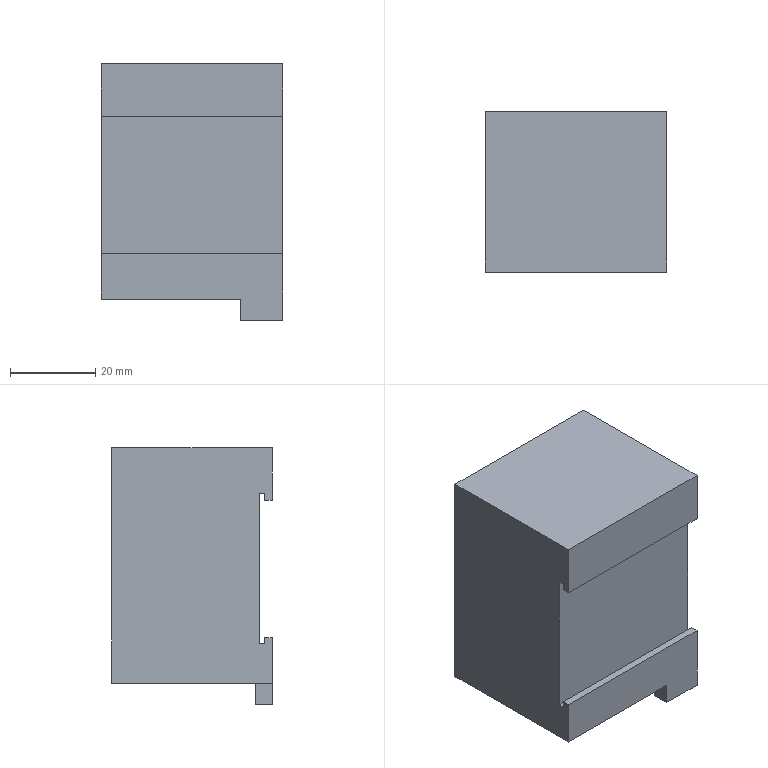Part | SolidWorks | features Cut 1, Extrusion 1, ICE 1 | 1 solid | 17 faces | box 42.7 x 37.7 x 60.3 mm | volume 84935 mm3 | plane 17
STEP:
#1=CARTESIAN_POINT('',(-21.35,0.,15.25));
#2=VERTEX_POINT('',#1);
#3=CARTESIAN_POINT('',(-21.35,0.,27.65));
#4=VERTEX_POINT('',#3);
#5=CARTESIAN_POINT('',(-21.35,0.,27.65));
#6=DIRECTION('',(0.,0.,1.));
#7=VECTOR('',#6,1000.);
#8=LINE('',#5,#7);
#9=EDGE_CURVE('',#2,#4,#8,.T.);
#10=ORIENTED_EDGE('',*,*,#9,.F.);
#11=CARTESIAN_POINT('',(21.35,0.,15.25));
#12=VERTEX_POINT('',#11);
#13=CARTESIAN_POINT('',(-21.351,0.,15.25));
#14=DIRECTION('',(1.,0.,0.));
#15=VECTOR('',#14,1000.);
#16=LINE('',#13,#15);
#17=EDGE_CURVE('',#2,#12,#16,.T.);
#18=ORIENTED_EDGE('',*,*,#17,.T.);
#19=CARTESIAN_POINT('',(21.35,0.,27.65));
#20=VERTEX_POINT('',#19);
#21=CARTESIAN_POINT('',(21.35,0.,27.65));
#22=DIRECTION('',(0.,0.,-1.));
#23=VECTOR('',#22,1000.);
#24=LINE('',#21,#23);
#25=EDGE_CURVE('',#20,#12,#24,.T.);
#26=ORIENTED_EDGE('',*,*,#25,.F.);
#27=CARTESIAN_POINT('',(-21.35,0.,27.65));
#28=DIRECTION('',(1.,0.,0.));
#29=VECTOR('',#28,1000.);
#30=LINE('',#27,#29);
#31=EDGE_CURVE('',#4,#20,#30,.T.);
#32=ORIENTED_EDGE('',*,*,#31,.F.);
#33=EDGE_LOOP('',(#10,#18,#26,#32));
#34=FACE_OUTER_BOUND('',#33,.T.);
#35=CARTESIAN_POINT('',(0.,0.,0.));
#36=DIRECTION('',(0.,-1.,0.));
#37=DIRECTION('',(0.,0.,-1.));
#38=AXIS2_PLACEMENT_3D('',#35,#36,#37);
#39=PLANE('',#38);
#40=ADVANCED_FACE('',(#34),#39,.T.);
#41=CARTESIAN_POINT('',(21.35,0.,-16.95));
#42=VERTEX_POINT('',#41);
#43=CARTESIAN_POINT('',(21.35,1.8,-16.95));
#44=VERTEX_POINT('',#43);
#45=CARTESIAN_POINT('',(21.35,1.8,-16.95));
#46=DIRECTION('',(0.,1.,0.));
#47=VECTOR('',#46,1000.);
#48=LINE('',#45,#47);
#49=EDGE_CURVE('',#42,#44,#48,.T.);
#50=ORIENTED_EDGE('',*,*,#49,.F.);
#51=CARTESIAN_POINT('',(21.35,0.,-32.65));
#52=VERTEX_POINT('',#51);
#53=CARTESIAN_POINT('',(21.35,0.,27.65));
#54=DIRECTION('',(0.,0.,-1.));
#55=VECTOR('',#54,1000.);
#56=LINE('',#53,#55);
#57=EDGE_CURVE('',#42,#52,#56,.T.);
#58=ORIENTED_EDGE('',*,*,#57,.T.);
#59=CARTESIAN_POINT('',(21.35,4.,-32.65));
#60=VERTEX_POINT('',#59);
#61=CARTESIAN_POINT('',(21.35,4.,-32.65));
#62=DIRECTION('',(0.,-1.,0.));
#63=VECTOR('',#62,1000.);
#64=LINE('',#61,#63);
#65=EDGE_CURVE('',#60,#52,#64,.T.);
#66=ORIENTED_EDGE('',*,*,#65,.F.);
#67=CARTESIAN_POINT('',(21.35,4.,-27.65));
#68=VERTEX_POINT('',#67);
#69=CARTESIAN_POINT('',(21.35,4.,-27.65));
#70=DIRECTION('',(0.,0.,1.));
#71=VECTOR('',#70,1000.);
#72=LINE('',#69,#71);
#73=EDGE_CURVE('',#60,#68,#72,.T.);
#74=ORIENTED_EDGE('',*,*,#73,.T.);
#75=CARTESIAN_POINT('',(21.35,37.7,-27.65));
#76=VERTEX_POINT('',#75);
#77=CARTESIAN_POINT('',(21.35,37.7,-27.65));
#78=DIRECTION('',(0.,-1.,0.));
#79=VECTOR('',#78,1000.);
#80=LINE('',#77,#79);
#81=EDGE_CURVE('',#76,#68,#80,.T.);
#82=ORIENTED_EDGE('',*,*,#81,.F.);
#83=CARTESIAN_POINT('',(21.35,37.7,27.65));
#84=VERTEX_POINT('',#83);
#85=CARTESIAN_POINT('',(21.35,37.7,27.65));
#86=DIRECTION('',(0.,0.,-1.));
#87=VECTOR('',#86,1000.);
#88=LINE('',#85,#87);
#89=EDGE_CURVE('',#84,#76,#88,.T.);
#90=ORIENTED_EDGE('',*,*,#89,.F.);
#91=CARTESIAN_POINT('',(21.35,37.7,27.65));
#92=DIRECTION('',(0.,-1.,0.));
#93=VECTOR('',#92,1000.);
#94=LINE('',#91,#93);
#95=EDGE_CURVE('',#84,#20,#94,.T.);
#96=ORIENTED_EDGE('',*,*,#95,.T.);
#97=ORIENTED_EDGE('',*,*,#25,.T.);
#98=CARTESIAN_POINT('',(21.35,1.8,15.25));
#99=VERTEX_POINT('',#98);
#100=CARTESIAN_POINT('',(21.35,0.,15.25));
#101=DIRECTION('',(0.,-1.,0.));
#102=VECTOR('',#101,1000.);
#103=LINE('',#100,#102);
#104=EDGE_CURVE('',#99,#12,#103,.T.);
#105=ORIENTED_EDGE('',*,*,#104,.F.);
#106=CARTESIAN_POINT('',(21.35,1.8,16.95));
#107=VERTEX_POINT('',#106);
#108=CARTESIAN_POINT('',(21.35,1.8,15.25));
#109=DIRECTION('',(0.,0.,-1.));
#110=VECTOR('',#109,1000.);
#111=LINE('',#108,#110);
#112=EDGE_CURVE('',#107,#99,#111,.T.);
#113=ORIENTED_EDGE('',*,*,#112,.F.);
#114=CARTESIAN_POINT('',(21.35,3.,16.95));
#115=VERTEX_POINT('',#114);
#116=CARTESIAN_POINT('',(21.35,1.8,16.95));
#117=DIRECTION('',(0.,-1.,0.));
#118=VECTOR('',#117,1000.);
#119=LINE('',#116,#118);
#120=EDGE_CURVE('',#115,#107,#119,.T.);
#121=ORIENTED_EDGE('',*,*,#120,.F.);
#122=CARTESIAN_POINT('',(21.35,3.,-18.4));
#123=VERTEX_POINT('',#122);
#124=CARTESIAN_POINT('',(21.35,3.,16.95));
#125=DIRECTION('',(0.,0.,1.));
#126=VECTOR('',#125,1000.);
#127=LINE('',#124,#126);
#128=EDGE_CURVE('',#123,#115,#127,.T.);
#129=ORIENTED_EDGE('',*,*,#128,.F.);
#130=CARTESIAN_POINT('',(21.35,1.8,-18.4));
#131=VERTEX_POINT('',#130);
#132=CARTESIAN_POINT('',(21.35,3.,-18.4));
#133=DIRECTION('',(0.,1.,0.));
#134=VECTOR('',#133,1000.);
#135=LINE('',#132,#134);
#136=EDGE_CURVE('',#131,#123,#135,.T.);
#137=ORIENTED_EDGE('',*,*,#136,.F.);
#138=CARTESIAN_POINT('',(21.35,1.8,-18.4));
#139=DIRECTION('',(0.,0.,-1.));
#140=VECTOR('',#139,1000.);
#141=LINE('',#138,#140);
#142=EDGE_CURVE('',#44,#131,#141,.T.);
#143=ORIENTED_EDGE('',*,*,#142,.F.);
#144=EDGE_LOOP('',(#50,#58,#66,#74,#82,#90,#96,#97,#105,#113,#121,#129,#137,#143));
#145=FACE_OUTER_BOUND('',#144,.T.);
#146=CARTESIAN_POINT('',(21.35,37.7,27.65));
#147=DIRECTION('',(-1.,0.,0.));
#148=DIRECTION('',(0.,0.,1.));
#149=AXIS2_PLACEMENT_3D('',#146,#147,#148);
#150=PLANE('',#149);
#151=ADVANCED_FACE('',(#145),#150,.F.);
#152=CARTESIAN_POINT('',(-21.35,1.8,15.25));
#153=VERTEX_POINT('',#152);
#154=CARTESIAN_POINT('',(-21.35,0.,15.25));
#155=DIRECTION('',(0.,1.,0.));
#156=VECTOR('',#155,1000.);
#157=LINE('',#154,#156);
#158=EDGE_CURVE('',#2,#153,#157,.T.);
#159=ORIENTED_EDGE('',*,*,#158,.F.);
#160=ORIENTED_EDGE('',*,*,#9,.T.);
#161=CARTESIAN_POINT('',(-21.35,37.7,27.65));
#162=VERTEX_POINT('',#161);
#163=CARTESIAN_POINT('',(-21.35,37.7,27.65));
#164=DIRECTION('',(0.,-1.,0.));
#165=VECTOR('',#164,1000.);
#166=LINE('',#163,#165);
#167=EDGE_CURVE('',#162,#4,#166,.T.);
#168=ORIENTED_EDGE('',*,*,#167,.F.);
#169=CARTESIAN_POINT('',(-21.35,37.7,-27.65));
#170=VERTEX_POINT('',#169);
#171=CARTESIAN_POINT('',(-21.35,37.7,27.65));
#172=DIRECTION('',(0.,0.,1.));
#173=VECTOR('',#172,1000.);
#174=LINE('',#171,#173);
#175=EDGE_CURVE('',#170,#162,#174,.T.);
#176=ORIENTED_EDGE('',*,*,#175,.F.);
#177=CARTESIAN_POINT('',(-21.35,0.,-27.65));
#178=VERTEX_POINT('',#177);
#179=CARTESIAN_POINT('',(-21.35,37.7,-27.65));
#180=DIRECTION('',(0.,-1.,0.));
#181=VECTOR('',#180,1000.);
#182=LINE('',#179,#181);
#183=EDGE_CURVE('',#170,#178,#182,.T.);
#184=ORIENTED_EDGE('',*,*,#183,.T.);
#185=CARTESIAN_POINT('',(-21.35,0.,-16.95));
#186=VERTEX_POINT('',#185);
#187=CARTESIAN_POINT('',(-21.35,0.,27.65));
#188=DIRECTION('',(0.,0.,1.));
#189=VECTOR('',#188,1000.);
#190=LINE('',#187,#189);
#191=EDGE_CURVE('',#178,#186,#190,.T.);
#192=ORIENTED_EDGE('',*,*,#191,.T.);
#193=CARTESIAN_POINT('',(-21.35,1.8,-16.95));
#194=VERTEX_POINT('',#193);
#195=CARTESIAN_POINT('',(-21.35,1.8,-16.95));
#196=DIRECTION('',(0.,-1.,0.));
#197=VECTOR('',#196,1000.);
#198=LINE('',#195,#197);
#199=EDGE_CURVE('',#194,#186,#198,.T.);
#200=ORIENTED_EDGE('',*,*,#199,.F.);
#201=CARTESIAN_POINT('',(-21.35,1.8,-18.4));
#202=VERTEX_POINT('',#201);
#203=CARTESIAN_POINT('',(-21.35,1.8,-18.4));
#204=DIRECTION('',(0.,0.,1.));
#205=VECTOR('',#204,1000.);
#206=LINE('',#203,#205);
#207=EDGE_CURVE('',#202,#194,#206,.T.);
#208=ORIENTED_EDGE('',*,*,#207,.F.);
#209=CARTESIAN_POINT('',(-21.35,3.,-18.4));
#210=VERTEX_POINT('',#209);
#211=CARTESIAN_POINT('',(-21.35,3.,-18.4));
#212=DIRECTION('',(0.,-1.,0.));
#213=VECTOR('',#212,1000.);
#214=LINE('',#211,#213);
#215=EDGE_CURVE('',#210,#202,#214,.T.);
#216=ORIENTED_EDGE('',*,*,#215,.F.);
#217=CARTESIAN_POINT('',(-21.35,3.,16.95));
#218=VERTEX_POINT('',#217);
#219=CARTESIAN_POINT('',(-21.35,3.,16.95));
#220=DIRECTION('',(0.,0.,-1.));
#221=VECTOR('',#220,1000.);
#222=LINE('',#219,#221);
#223=EDGE_CURVE('',#218,#210,#222,.T.);
#224=ORIENTED_EDGE('',*,*,#223,.F.);
#225=CARTESIAN_POINT('',(-21.35,1.8,16.95));
#226=VERTEX_POINT('',#225);
#227=CARTESIAN_POINT('',(-21.35,1.8,16.95));
#228=DIRECTION('',(0.,1.,0.));
#229=VECTOR('',#228,1000.);
#230=LINE('',#227,#229);
#231=EDGE_CURVE('',#226,#218,#230,.T.);
#232=ORIENTED_EDGE('',*,*,#231,.F.);
#233=CARTESIAN_POINT('',(-21.35,1.8,15.25));
#234=DIRECTION('',(0.,0.,1.));
#235=VECTOR('',#234,1000.);
#236=LINE('',#233,#235);
#237=EDGE_CURVE('',#153,#226,#236,.T.);
#238=ORIENTED_EDGE('',*,*,#237,.F.);
#239=EDGE_LOOP('',(#159,#160,#168,#176,#184,#192,#200,#208,#216,#224,#232,#238));
#240=FACE_OUTER_BOUND('',#239,.T.);
#241=CARTESIAN_POINT('',(-21.35,37.7,27.65));
#242=DIRECTION('',(1.,0.,0.));
#243=DIRECTION('',(0.,0.,-1.));
#244=AXIS2_PLACEMENT_3D('',#241,#242,#243);
#245=PLANE('',#244);
#246=ADVANCED_FACE('',(#240),#245,.F.);
#247=ORIENTED_EDGE('',*,*,#81,.T.);
#248=CARTESIAN_POINT('',(11.35,4.,-27.65));
#249=VERTEX_POINT('',#248);
#250=CARTESIAN_POINT('',(21.35,4.,-27.65));
#251=DIRECTION('',(-1.,0.,0.));
#252=VECTOR('',#251,1000.);
#253=LINE('',#250,#252);
#254=EDGE_CURVE('',#68,#249,#253,.T.);
#255=ORIENTED_EDGE('',*,*,#254,.T.);
#256=CARTESIAN_POINT('',(11.35,0.,-27.65));
#257=VERTEX_POINT('',#256);
#258=CARTESIAN_POINT('',(11.35,4.,-27.65));
#259=DIRECTION('',(0.,-1.,0.));
#260=VECTOR('',#259,1000.);
#261=LINE('',#258,#260);
#262=EDGE_CURVE('',#249,#257,#261,.T.);
#263=ORIENTED_EDGE('',*,*,#262,.T.);
#264=CARTESIAN_POINT('',(-21.35,0.,-27.65));
#265=DIRECTION('',(-1.,0.,0.));
#266=VECTOR('',#265,1000.);
#267=LINE('',#264,#266);
#268=EDGE_CURVE('',#257,#178,#267,.T.);
#269=ORIENTED_EDGE('',*,*,#268,.T.);
#270=ORIENTED_EDGE('',*,*,#183,.F.);
#271=CARTESIAN_POINT('',(-21.35,37.7,-27.65));
#272=DIRECTION('',(-1.,0.,0.));
#273=VECTOR('',#272,1000.);
#274=LINE('',#271,#273);
#275=EDGE_CURVE('',#76,#170,#274,.T.);
#276=ORIENTED_EDGE('',*,*,#275,.F.);
#277=EDGE_LOOP('',(#247,#255,#263,#269,#270,#276));
#278=FACE_OUTER_BOUND('',#277,.T.);
#279=CARTESIAN_POINT('',(-21.35,37.7,-27.65));
#280=DIRECTION('',(0.,0.,1.));
#281=DIRECTION('',(1.,0.,0.));
#282=AXIS2_PLACEMENT_3D('',#279,#280,#281);
#283=PLANE('',#282);
#284=ADVANCED_FACE('',(#278),#283,.F.);
#285=ORIENTED_EDGE('',*,*,#31,.T.);
#286=ORIENTED_EDGE('',*,*,#95,.F.);
#287=CARTESIAN_POINT('',(-21.35,37.7,27.65));
#288=DIRECTION('',(1.,0.,0.));
#289=VECTOR('',#288,1000.);
#290=LINE('',#287,#289);
#291=EDGE_CURVE('',#162,#84,#290,.T.);
#292=ORIENTED_EDGE('',*,*,#291,.F.);
#293=ORIENTED_EDGE('',*,*,#167,.T.);
#294=EDGE_LOOP('',(#285,#286,#292,#293));
#295=FACE_OUTER_BOUND('',#294,.T.);
#296=CARTESIAN_POINT('',(-21.35,37.7,27.65));
#297=DIRECTION('',(0.,0.,-1.));
#298=DIRECTION('',(-1.,0.,0.));
#299=AXIS2_PLACEMENT_3D('',#296,#297,#298);
#300=PLANE('',#299);
#301=ADVANCED_FACE('',(#295),#300,.F.);
#302=ORIENTED_EDGE('',*,*,#89,.T.);
#303=ORIENTED_EDGE('',*,*,#275,.T.);
#304=ORIENTED_EDGE('',*,*,#175,.T.);
#305=ORIENTED_EDGE('',*,*,#291,.T.);
#306=EDGE_LOOP('',(#302,#303,#304,#305));
#307=FACE_OUTER_BOUND('',#306,.T.);
#308=CARTESIAN_POINT('',(0.,37.7,0.));
#309=DIRECTION('',(0.,-1.,0.));
#310=DIRECTION('',(0.,0.,-1.));
#311=AXIS2_PLACEMENT_3D('',#308,#309,#310);
#312=PLANE('',#311);
#313=ADVANCED_FACE('',(#307),#312,.F.);
#314=CARTESIAN_POINT('',(-21.351,0.,-16.95));
#315=DIRECTION('',(1.,0.,0.));
#316=VECTOR('',#315,1000.);
#317=LINE('',#314,#316);
#318=EDGE_CURVE('',#186,#42,#317,.T.);
#319=ORIENTED_EDGE('',*,*,#318,.F.);
#320=ORIENTED_EDGE('',*,*,#191,.F.);
#321=ORIENTED_EDGE('',*,*,#268,.F.);
#322=CARTESIAN_POINT('',(11.35,0.,-32.65));
#323=VERTEX_POINT('',#322);
#324=CARTESIAN_POINT('',(11.35,0.,-27.65));
#325=DIRECTION('',(0.,0.,-1.));
#326=VECTOR('',#325,1000.);
#327=LINE('',#324,#326);
#328=EDGE_CURVE('',#257,#323,#327,.T.);
#329=ORIENTED_EDGE('',*,*,#328,.T.);
#330=CARTESIAN_POINT('',(21.35,0.,-32.65));
#331=DIRECTION('',(1.,0.,0.));
#332=VECTOR('',#331,1000.);
#333=LINE('',#330,#332);
#334=EDGE_CURVE('',#323,#52,#333,.T.);
#335=ORIENTED_EDGE('',*,*,#334,.T.);
#336=ORIENTED_EDGE('',*,*,#57,.F.);
#337=EDGE_LOOP('',(#319,#320,#321,#329,#335,#336));
#338=FACE_OUTER_BOUND('',#337,.T.);
#339=CARTESIAN_POINT('',(0.,0.,0.));
#340=DIRECTION('',(0.,-1.,0.));
#341=DIRECTION('',(0.,0.,-1.));
#342=AXIS2_PLACEMENT_3D('',#339,#340,#341);
#343=PLANE('',#342);
#344=ADVANCED_FACE('',(#338),#343,.T.);
#345=ORIENTED_EDGE('',*,*,#158,.T.);
#346=CARTESIAN_POINT('',(-21.351,1.8,15.25));
#347=DIRECTION('',(1.,0.,0.));
#348=VECTOR('',#347,1000.);
#349=LINE('',#346,#348);
#350=EDGE_CURVE('',#153,#99,#349,.T.);
#351=ORIENTED_EDGE('',*,*,#350,.T.);
#352=ORIENTED_EDGE('',*,*,#104,.T.);
#353=ORIENTED_EDGE('',*,*,#17,.F.);
#354=EDGE_LOOP('',(#345,#351,#352,#353));
#355=FACE_OUTER_BOUND('',#354,.T.);
#356=CARTESIAN_POINT('',(-21.351,0.,15.25));
#357=DIRECTION('',(0.,0.,1.));
#358=DIRECTION('',(1.,0.,0.));
#359=AXIS2_PLACEMENT_3D('',#356,#357,#358);
#360=PLANE('',#359);
#361=ADVANCED_FACE('',(#355),#360,.F.);
#362=ORIENTED_EDGE('',*,*,#237,.T.);
#363=CARTESIAN_POINT('',(-21.351,1.8,16.95));
#364=DIRECTION('',(1.,0.,0.));
#365=VECTOR('',#364,1000.);
#366=LINE('',#363,#365);
#367=EDGE_CURVE('',#226,#107,#366,.T.);
#368=ORIENTED_EDGE('',*,*,#367,.T.);
#369=ORIENTED_EDGE('',*,*,#112,.T.);
#370=ORIENTED_EDGE('',*,*,#350,.F.);
#371=EDGE_LOOP('',(#362,#368,#369,#370));
#372=FACE_OUTER_BOUND('',#371,.T.);
#373=CARTESIAN_POINT('',(-21.351,1.8,15.25));
#374=DIRECTION('',(0.,-1.,0.));
#375=DIRECTION('',(0.,0.,-1.));
#376=AXIS2_PLACEMENT_3D('',#373,#374,#375);
#377=PLANE('',#376);
#378=ADVANCED_FACE('',(#372),#377,.F.);
#379=ORIENTED_EDGE('',*,*,#231,.T.);
#380=CARTESIAN_POINT('',(-21.351,3.,16.95));
#381=DIRECTION('',(1.,0.,0.));
#382=VECTOR('',#381,1000.);
#383=LINE('',#380,#382);
#384=EDGE_CURVE('',#218,#115,#383,.T.);
#385=ORIENTED_EDGE('',*,*,#384,.T.);
#386=ORIENTED_EDGE('',*,*,#120,.T.);
#387=ORIENTED_EDGE('',*,*,#367,.F.);
#388=EDGE_LOOP('',(#379,#385,#386,#387));
#389=FACE_OUTER_BOUND('',#388,.T.);
#390=CARTESIAN_POINT('',(-21.351,1.8,16.95));
#391=DIRECTION('',(0.,0.,1.));
#392=DIRECTION('',(1.,0.,0.));
#393=AXIS2_PLACEMENT_3D('',#390,#391,#392);
#394=PLANE('',#393);
#395=ADVANCED_FACE('',(#389),#394,.F.);
#396=ORIENTED_EDGE('',*,*,#223,.T.);
#397=CARTESIAN_POINT('',(-21.351,3.,-18.4));
#398=DIRECTION('',(1.,0.,0.));
#399=VECTOR('',#398,1000.);
#400=LINE('',#397,#399);
#401=EDGE_CURVE('',#210,#123,#400,.T.);
#402=ORIENTED_EDGE('',*,*,#401,.T.);
#403=ORIENTED_EDGE('',*,*,#128,.T.);
#404=ORIENTED_EDGE('',*,*,#384,.F.);
#405=EDGE_LOOP('',(#396,#402,#403,#404));
#406=FACE_OUTER_BOUND('',#405,.T.);
#407=CARTESIAN_POINT('',(-21.351,3.,16.95));
#408=DIRECTION('',(0.,1.,0.));
#409=DIRECTION('',(0.,0.,1.));
#410=AXIS2_PLACEMENT_3D('',#407,#408,#409);
#411=PLANE('',#410);
#412=ADVANCED_FACE('',(#406),#411,.F.);
#413=ORIENTED_EDGE('',*,*,#215,.T.);
#414=CARTESIAN_POINT('',(-21.351,1.8,-18.4));
#415=DIRECTION('',(1.,0.,0.));
#416=VECTOR('',#415,1000.);
#417=LINE('',#414,#416);
#418=EDGE_CURVE('',#202,#131,#417,.T.);
#419=ORIENTED_EDGE('',*,*,#418,.T.);
#420=ORIENTED_EDGE('',*,*,#136,.T.);
#421=ORIENTED_EDGE('',*,*,#401,.F.);
#422=EDGE_LOOP('',(#413,#419,#420,#421));
#423=FACE_OUTER_BOUND('',#422,.T.);
#424=CARTESIAN_POINT('',(-21.351,3.,-18.4));
#425=DIRECTION('',(0.,0.,-1.));
#426=DIRECTION('',(0.,1.,0.));
#427=AXIS2_PLACEMENT_3D('',#424,#425,#426);
#428=PLANE('',#427);
#429=ADVANCED_FACE('',(#423),#428,.F.);
#430=ORIENTED_EDGE('',*,*,#207,.T.);
#431=CARTESIAN_POINT('',(-21.351,1.8,-16.95));
#432=DIRECTION('',(1.,0.,0.));
#433=VECTOR('',#432,1000.);
#434=LINE('',#431,#433);
#435=EDGE_CURVE('',#194,#44,#434,.T.);
#436=ORIENTED_EDGE('',*,*,#435,.T.);
#437=ORIENTED_EDGE('',*,*,#142,.T.);
#438=ORIENTED_EDGE('',*,*,#418,.F.);
#439=EDGE_LOOP('',(#430,#436,#437,#438));
#440=FACE_OUTER_BOUND('',#439,.T.);
#441=CARTESIAN_POINT('',(-21.351,1.8,-18.4));
#442=DIRECTION('',(0.,-1.,0.));
#443=DIRECTION('',(0.,0.,-1.));
#444=AXIS2_PLACEMENT_3D('',#441,#442,#443);
#445=PLANE('',#444);
#446=ADVANCED_FACE('',(#440),#445,.F.);
#447=ORIENTED_EDGE('',*,*,#199,.T.);
#448=ORIENTED_EDGE('',*,*,#318,.T.);
#449=ORIENTED_EDGE('',*,*,#49,.T.);
#450=ORIENTED_EDGE('',*,*,#435,.F.);
#451=EDGE_LOOP('',(#447,#448,#449,#450));
#452=FACE_OUTER_BOUND('',#451,.T.);
#453=CARTESIAN_POINT('',(-21.351,1.8,-16.95));
#454=DIRECTION('',(0.,0.,-1.));
#455=DIRECTION('',(-1.,0.,0.));
#456=AXIS2_PLACEMENT_3D('',#453,#454,#455);
#457=PLANE('',#456);
#458=ADVANCED_FACE('',(#452),#457,.F.);
#459=ORIENTED_EDGE('',*,*,#334,.F.);
#460=CARTESIAN_POINT('',(11.35,4.,-32.65));
#461=VERTEX_POINT('',#460);
#462=CARTESIAN_POINT('',(11.35,4.,-32.65));
#463=DIRECTION('',(0.,-1.,0.));
#464=VECTOR('',#463,1000.);
#465=LINE('',#462,#464);
#466=EDGE_CURVE('',#461,#323,#465,.T.);
#467=ORIENTED_EDGE('',*,*,#466,.F.);
#468=CARTESIAN_POINT('',(21.35,4.,-32.65));
#469=DIRECTION('',(1.,0.,0.));
#470=VECTOR('',#469,1000.);
#471=LINE('',#468,#470);
#472=EDGE_CURVE('',#461,#60,#471,.T.);
#473=ORIENTED_EDGE('',*,*,#472,.T.);
#474=ORIENTED_EDGE('',*,*,#65,.T.);
#475=EDGE_LOOP('',(#459,#467,#473,#474));
#476=FACE_OUTER_BOUND('',#475,.T.);
#477=CARTESIAN_POINT('',(21.35,4.,-32.65));
#478=DIRECTION('',(0.,0.,-1.));
#479=DIRECTION('',(-1.,0.,0.));
#480=AXIS2_PLACEMENT_3D('',#477,#478,#479);
#481=PLANE('',#480);
#482=ADVANCED_FACE('',(#476),#481,.T.);
#483=ORIENTED_EDGE('',*,*,#328,.F.);
#484=ORIENTED_EDGE('',*,*,#262,.F.);
#485=CARTESIAN_POINT('',(11.35,4.,-27.65));
#486=DIRECTION('',(0.,0.,-1.));
#487=VECTOR('',#486,1000.);
#488=LINE('',#485,#487);
#489=EDGE_CURVE('',#249,#461,#488,.T.);
#490=ORIENTED_EDGE('',*,*,#489,.T.);
#491=ORIENTED_EDGE('',*,*,#466,.T.);
#492=EDGE_LOOP('',(#483,#484,#490,#491));
#493=FACE_OUTER_BOUND('',#492,.T.);
#494=CARTESIAN_POINT('',(11.35,4.,-27.65));
#495=DIRECTION('',(-1.,0.,0.));
#496=DIRECTION('',(0.,0.,1.));
#497=AXIS2_PLACEMENT_3D('',#494,#495,#496);
#498=PLANE('',#497);
#499=ADVANCED_FACE('',(#493),#498,.T.);
#500=ORIENTED_EDGE('',*,*,#73,.F.);
#501=ORIENTED_EDGE('',*,*,#472,.F.);
#502=ORIENTED_EDGE('',*,*,#489,.F.);
#503=ORIENTED_EDGE('',*,*,#254,.F.);
#504=EDGE_LOOP('',(#500,#501,#502,#503));
#505=FACE_OUTER_BOUND('',#504,.T.);
#506=CARTESIAN_POINT('',(0.,4.,0.));
#507=DIRECTION('',(0.,1.,0.));
#508=DIRECTION('',(0.,0.,1.));
#509=AXIS2_PLACEMENT_3D('',#506,#507,#508);
#510=PLANE('',#509);
#511=ADVANCED_FACE('',(#505),#510,.T.);
#512=CLOSED_SHELL('',(#40,#151,#246,#284,#301,#313,#344,#361,#378,#395,#412,#429,#446,#458,#482,#499,#511));
#513=MANIFOLD_SOLID_BREP('',#512);
#514=CARTESIAN_POINT('',(0.,0.,0.));
#515=DIRECTION('',(0.,0.,1.));
#516=DIRECTION('',(1.,0.,0.));
#517=AXIS2_PLACEMENT_3D('',#514,#515,#516);
#518=(LENGTH_UNIT()NAMED_UNIT(*)SI_UNIT(.MILLI.,.METRE.));
#519=UNCERTAINTY_MEASURE_WITH_UNIT(LENGTH_MEASURE(0.00001),#518,'','');
#520=(NAMED_UNIT(*)PLANE_ANGLE_UNIT()SI_UNIT($,.RADIAN.));
#521=(NAMED_UNIT(*)SI_UNIT($,.STERADIAN.)SOLID_ANGLE_UNIT());
#522=(GEOMETRIC_REPRESENTATION_CONTEXT(3)GLOBAL_UNCERTAINTY_ASSIGNED_CONTEXT((#519))GLOBAL_UNIT_ASSIGNED_CONTEXT((#518,#520,#521))REPRESENTATION_CONTEXT('',''));
#523=ADVANCED_BREP_SHAPE_REPRESENTATION('',(#513,#517),#522);